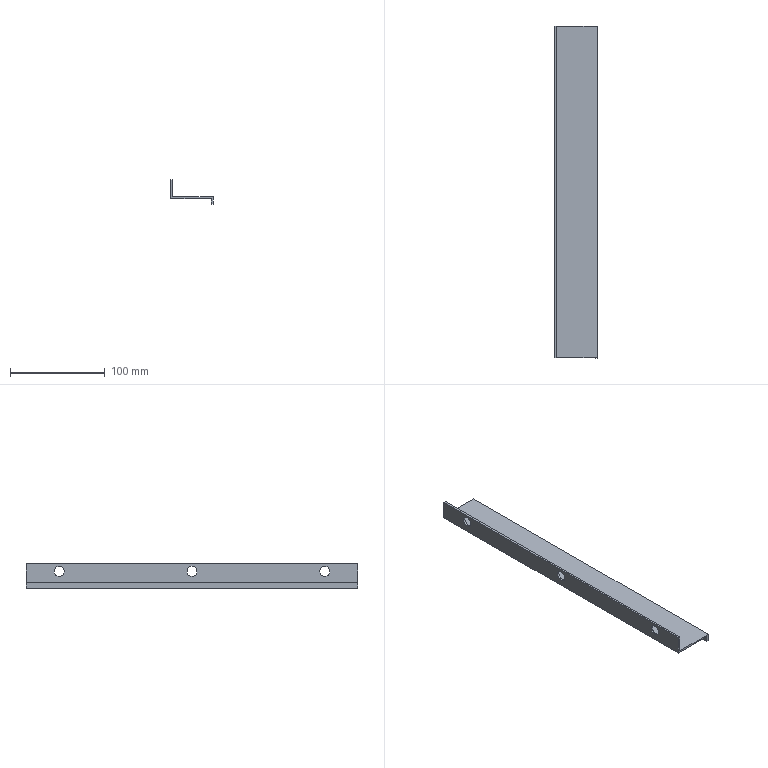Part | SolidWorks | features BaseBody 1 | 1 solid | 16 faces | box 44.5 x 350 x 26 mm | volume 47421 mm3 | plane 10 | cylinder 6 | commonest cylinder face diameters 10.6 x6
STEP:
#1=CARTESIAN_POINT('',(236.946,-4310.973,1968.771));
#2=VERTEX_POINT('',#1);
#3=CARTESIAN_POINT('',(236.946,-4310.973,1958.171));
#4=VERTEX_POINT('',#3);
#5=CARTESIAN_POINT('',(236.946,-4310.973,1963.471));
#6=DIRECTION('',(1.,0.,0.));
#7=DIRECTION('',(0.,0.,-1.));
#8=AXIS2_PLACEMENT_3D('',#5,#6,#7);
#9=CIRCLE('',#8,5.3);
#10=EDGE_CURVE('',#2,#4,#9,.T.);
#11=ORIENTED_EDGE('',*,*,#10,.F.);
#12=CARTESIAN_POINT('',(238.946,-4310.973,1968.771));
#13=VERTEX_POINT('',#12);
#14=CARTESIAN_POINT('',(270.923,-4310.973,1968.771));
#15=DIRECTION('',(1.,0.,0.));
#16=VECTOR('',#15,1000.);
#17=LINE('',#14,#16);
#18=EDGE_CURVE('',#2,#13,#17,.T.);
#19=ORIENTED_EDGE('',*,*,#18,.T.);
#20=CARTESIAN_POINT('',(238.946,-4310.973,1958.171));
#21=VERTEX_POINT('',#20);
#22=CARTESIAN_POINT('',(238.946,-4310.973,1963.471));
#23=DIRECTION('',(-1.,0.,0.));
#24=DIRECTION('',(0.,0.,-1.));
#25=AXIS2_PLACEMENT_3D('',#22,#23,#24);
#26=CIRCLE('',#25,5.3);
#27=EDGE_CURVE('',#21,#13,#26,.T.);
#28=ORIENTED_EDGE('',*,*,#27,.F.);
#29=CARTESIAN_POINT('',(270.923,-4310.973,1958.171));
#30=DIRECTION('',(1.,0.,0.));
#31=VECTOR('',#30,1000.);
#32=LINE('',#29,#31);
#33=EDGE_CURVE('',#4,#21,#32,.T.);
#34=ORIENTED_EDGE('',*,*,#33,.F.);
#35=EDGE_LOOP('',(#11,#19,#28,#34));
#36=FACE_OUTER_BOUND('',#35,.T.);
#37=CARTESIAN_POINT('',(270.923,-4310.973,1963.471));
#38=DIRECTION('',(1.,0.,0.));
#39=DIRECTION('',(0.,0.,-1.));
#40=AXIS2_PLACEMENT_3D('',#37,#38,#39);
#41=CYLINDRICAL_SURFACE('',#40,5.3);
#42=ADVANCED_FACE('',(#36),#41,.F.);
#43=CARTESIAN_POINT('',(236.946,-4030.973,1968.771));
#44=VERTEX_POINT('',#43);
#45=CARTESIAN_POINT('',(236.946,-4030.973,1958.171));
#46=VERTEX_POINT('',#45);
#47=CARTESIAN_POINT('',(236.946,-4030.973,1963.471));
#48=DIRECTION('',(1.,0.,0.));
#49=DIRECTION('',(0.,0.,-1.));
#50=AXIS2_PLACEMENT_3D('',#47,#48,#49);
#51=CIRCLE('',#50,5.3);
#52=EDGE_CURVE('',#44,#46,#51,.T.);
#53=ORIENTED_EDGE('',*,*,#52,.F.);
#54=CARTESIAN_POINT('',(238.946,-4030.973,1968.771));
#55=VERTEX_POINT('',#54);
#56=CARTESIAN_POINT('',(270.923,-4030.973,1968.771));
#57=DIRECTION('',(1.,0.,0.));
#58=VECTOR('',#57,1000.);
#59=LINE('',#56,#58);
#60=EDGE_CURVE('',#44,#55,#59,.T.);
#61=ORIENTED_EDGE('',*,*,#60,.T.);
#62=CARTESIAN_POINT('',(238.946,-4030.973,1958.171));
#63=VERTEX_POINT('',#62);
#64=CARTESIAN_POINT('',(238.946,-4030.973,1963.471));
#65=DIRECTION('',(-1.,0.,0.));
#66=DIRECTION('',(0.,0.,-1.));
#67=AXIS2_PLACEMENT_3D('',#64,#65,#66);
#68=CIRCLE('',#67,5.3);
#69=EDGE_CURVE('',#63,#55,#68,.T.);
#70=ORIENTED_EDGE('',*,*,#69,.F.);
#71=CARTESIAN_POINT('',(270.923,-4030.973,1958.171));
#72=DIRECTION('',(1.,0.,0.));
#73=VECTOR('',#72,1000.);
#74=LINE('',#71,#73);
#75=EDGE_CURVE('',#46,#63,#74,.T.);
#76=ORIENTED_EDGE('',*,*,#75,.F.);
#77=EDGE_LOOP('',(#53,#61,#70,#76));
#78=FACE_OUTER_BOUND('',#77,.T.);
#79=CARTESIAN_POINT('',(270.923,-4030.973,1963.471));
#80=DIRECTION('',(1.,0.,0.));
#81=DIRECTION('',(0.,0.,-1.));
#82=AXIS2_PLACEMENT_3D('',#79,#80,#81);
#83=CYLINDRICAL_SURFACE('',#82,5.3);
#84=ADVANCED_FACE('',(#78),#83,.F.);
#85=CARTESIAN_POINT('',(236.946,-4170.973,1968.771));
#86=VERTEX_POINT('',#85);
#87=CARTESIAN_POINT('',(236.946,-4170.973,1958.171));
#88=VERTEX_POINT('',#87);
#89=CARTESIAN_POINT('',(236.946,-4170.973,1963.471));
#90=DIRECTION('',(1.,0.,0.));
#91=DIRECTION('',(0.,0.,-1.));
#92=AXIS2_PLACEMENT_3D('',#89,#90,#91);
#93=CIRCLE('',#92,5.3);
#94=EDGE_CURVE('',#86,#88,#93,.T.);
#95=ORIENTED_EDGE('',*,*,#94,.F.);
#96=CARTESIAN_POINT('',(238.946,-4170.973,1968.771));
#97=VERTEX_POINT('',#96);
#98=CARTESIAN_POINT('',(270.923,-4170.973,1968.771));
#99=DIRECTION('',(1.,0.,0.));
#100=VECTOR('',#99,1000.);
#101=LINE('',#98,#100);
#102=EDGE_CURVE('',#86,#97,#101,.T.);
#103=ORIENTED_EDGE('',*,*,#102,.T.);
#104=CARTESIAN_POINT('',(238.946,-4170.973,1958.171));
#105=VERTEX_POINT('',#104);
#106=CARTESIAN_POINT('',(238.946,-4170.973,1963.471));
#107=DIRECTION('',(-1.,0.,0.));
#108=DIRECTION('',(0.,0.,-1.));
#109=AXIS2_PLACEMENT_3D('',#106,#107,#108);
#110=CIRCLE('',#109,5.3);
#111=EDGE_CURVE('',#105,#97,#110,.T.);
#112=ORIENTED_EDGE('',*,*,#111,.F.);
#113=CARTESIAN_POINT('',(270.923,-4170.973,1958.171));
#114=DIRECTION('',(1.,0.,0.));
#115=VECTOR('',#114,1000.);
#116=LINE('',#113,#115);
#117=EDGE_CURVE('',#88,#105,#116,.T.);
#118=ORIENTED_EDGE('',*,*,#117,.F.);
#119=EDGE_LOOP('',(#95,#103,#112,#118));
#120=FACE_OUTER_BOUND('',#119,.T.);
#121=CARTESIAN_POINT('',(270.923,-4170.973,1963.471));
#122=DIRECTION('',(1.,0.,0.));
#123=DIRECTION('',(0.,0.,-1.));
#124=AXIS2_PLACEMENT_3D('',#121,#122,#123);
#125=CYLINDRICAL_SURFACE('',#124,5.3);
#126=ADVANCED_FACE('',(#120),#125,.F.);
#127=CARTESIAN_POINT('',(236.946,-3995.973,1951.471));
#128=VERTEX_POINT('',#127);
#129=CARTESIAN_POINT('',(279.446,-3995.973,1951.471));
#130=VERTEX_POINT('',#129);
#131=CARTESIAN_POINT('',(277.446,-3995.973,1951.471));
#132=DIRECTION('',(1.,0.,0.));
#133=VECTOR('',#132,1000.);
#134=LINE('',#131,#133);
#135=EDGE_CURVE('',#128,#130,#134,.T.);
#136=ORIENTED_EDGE('',*,*,#135,.T.);
#137=CARTESIAN_POINT('',(279.446,-4345.973,1951.471));
#138=VERTEX_POINT('',#137);
#139=CARTESIAN_POINT('',(279.446,-3995.973,1951.471));
#140=DIRECTION('',(0.,-1.,0.));
#141=VECTOR('',#140,1000.);
#142=LINE('',#139,#141);
#143=EDGE_CURVE('',#130,#138,#142,.T.);
#144=ORIENTED_EDGE('',*,*,#143,.T.);
#145=CARTESIAN_POINT('',(236.946,-4345.973,1951.471));
#146=VERTEX_POINT('',#145);
#147=CARTESIAN_POINT('',(277.446,-4345.973,1951.471));
#148=DIRECTION('',(-1.,0.,0.));
#149=VECTOR('',#148,1000.);
#150=LINE('',#147,#149);
#151=EDGE_CURVE('',#138,#146,#150,.T.);
#152=ORIENTED_EDGE('',*,*,#151,.T.);
#153=CARTESIAN_POINT('',(236.946,-3995.973,1951.471));
#154=DIRECTION('',(0.,1.,0.));
#155=VECTOR('',#154,1000.);
#156=LINE('',#153,#155);
#157=EDGE_CURVE('',#146,#128,#156,.T.);
#158=ORIENTED_EDGE('',*,*,#157,.T.);
#159=EDGE_LOOP('',(#136,#144,#152,#158));
#160=FACE_OUTER_BOUND('',#159,.T.);
#161=CARTESIAN_POINT('',(277.446,-3995.973,1951.471));
#162=DIRECTION('',(0.,0.,-1.));
#163=DIRECTION('',(-1.,0.,0.));
#164=AXIS2_PLACEMENT_3D('',#161,#162,#163);
#165=PLANE('',#164);
#166=ADVANCED_FACE('',(#160),#165,.T.);
#167=CARTESIAN_POINT('',(279.446,-3995.973,1945.471));
#168=VERTEX_POINT('',#167);
#169=CARTESIAN_POINT('',(279.446,-3995.973,1945.471));
#170=DIRECTION('',(0.,0.,-1.));
#171=VECTOR('',#170,1000.);
#172=LINE('',#169,#171);
#173=EDGE_CURVE('',#130,#168,#172,.T.);
#174=ORIENTED_EDGE('',*,*,#173,.T.);
#175=CARTESIAN_POINT('',(279.446,-4345.973,1945.471));
#176=VERTEX_POINT('',#175);
#177=CARTESIAN_POINT('',(279.446,-3995.973,1945.471));
#178=DIRECTION('',(0.,-1.,0.));
#179=VECTOR('',#178,1000.);
#180=LINE('',#177,#179);
#181=EDGE_CURVE('',#168,#176,#180,.T.);
#182=ORIENTED_EDGE('',*,*,#181,.T.);
#183=CARTESIAN_POINT('',(279.446,-4345.973,1945.471));
#184=DIRECTION('',(0.,0.,1.));
#185=VECTOR('',#184,1000.);
#186=LINE('',#183,#185);
#187=EDGE_CURVE('',#176,#138,#186,.T.);
#188=ORIENTED_EDGE('',*,*,#187,.T.);
#189=ORIENTED_EDGE('',*,*,#143,.F.);
#190=EDGE_LOOP('',(#174,#182,#188,#189));
#191=FACE_OUTER_BOUND('',#190,.T.);
#192=CARTESIAN_POINT('',(279.446,-3995.973,1945.471));
#193=DIRECTION('',(-1.,0.,0.));
#194=DIRECTION('',(0.,0.,1.));
#195=AXIS2_PLACEMENT_3D('',#192,#193,#194);
#196=PLANE('',#195);
#197=ADVANCED_FACE('',(#191),#196,.T.);
#198=CARTESIAN_POINT('',(236.946,-3995.973,1971.471));
#199=VERTEX_POINT('',#198);
#200=CARTESIAN_POINT('',(236.946,-3995.973,1956.835));
#201=DIRECTION('',(0.,0.,1.));
#202=VECTOR('',#201,1000.);
#203=LINE('',#200,#202);
#204=EDGE_CURVE('',#128,#199,#203,.T.);
#205=ORIENTED_EDGE('',*,*,#204,.T.);
#206=CARTESIAN_POINT('',(238.946,-3995.973,1971.471));
#207=VERTEX_POINT('',#206);
#208=CARTESIAN_POINT('',(271.559,-3995.973,1971.471));
#209=DIRECTION('',(1.,0.,0.));
#210=VECTOR('',#209,1000.);
#211=LINE('',#208,#210);
#212=EDGE_CURVE('',#199,#207,#211,.T.);
#213=ORIENTED_EDGE('',*,*,#212,.T.);
#214=CARTESIAN_POINT('',(238.946,-3995.973,1953.471));
#215=VERTEX_POINT('',#214);
#216=CARTESIAN_POINT('',(238.946,-3995.973,1956.835));
#217=DIRECTION('',(0.,0.,-1.));
#218=VECTOR('',#217,1000.);
#219=LINE('',#216,#218);
#220=EDGE_CURVE('',#207,#215,#219,.T.);
#221=ORIENTED_EDGE('',*,*,#220,.T.);
#222=CARTESIAN_POINT('',(281.446,-3995.973,1953.471));
#223=VERTEX_POINT('',#222);
#224=CARTESIAN_POINT('',(271.559,-3995.973,1953.471));
#225=DIRECTION('',(1.,0.,0.));
#226=VECTOR('',#225,1000.);
#227=LINE('',#224,#226);
#228=EDGE_CURVE('',#215,#223,#227,.T.);
#229=ORIENTED_EDGE('',*,*,#228,.T.);
#230=CARTESIAN_POINT('',(281.446,-3995.973,1945.471));
#231=VERTEX_POINT('',#230);
#232=CARTESIAN_POINT('',(281.446,-3995.973,1956.835));
#233=DIRECTION('',(0.,0.,-1.));
#234=VECTOR('',#233,1000.);
#235=LINE('',#232,#234);
#236=EDGE_CURVE('',#223,#231,#235,.T.);
#237=ORIENTED_EDGE('',*,*,#236,.T.);
#238=CARTESIAN_POINT('',(271.559,-3995.973,1945.471));
#239=DIRECTION('',(-1.,0.,0.));
#240=VECTOR('',#239,1000.);
#241=LINE('',#238,#240);
#242=EDGE_CURVE('',#231,#168,#241,.T.);
#243=ORIENTED_EDGE('',*,*,#242,.T.);
#244=ORIENTED_EDGE('',*,*,#173,.F.);
#245=ORIENTED_EDGE('',*,*,#135,.F.);
#246=EDGE_LOOP('',(#205,#213,#221,#229,#237,#243,#244,#245));
#247=FACE_OUTER_BOUND('',#246,.T.);
#248=CARTESIAN_POINT('',(271.559,-3995.973,1956.835));
#249=DIRECTION('',(0.,1.,0.));
#250=DIRECTION('',(0.,0.,1.));
#251=AXIS2_PLACEMENT_3D('',#248,#249,#250);
#252=PLANE('',#251);
#253=ADVANCED_FACE('',(#247),#252,.T.);
#254=ORIENTED_EDGE('',*,*,#204,.F.);
#255=ORIENTED_EDGE('',*,*,#157,.F.);
#256=CARTESIAN_POINT('',(236.946,-4345.973,1971.471));
#257=VERTEX_POINT('',#256);
#258=CARTESIAN_POINT('',(236.946,-4345.973,1951.471));
#259=DIRECTION('',(0.,0.,1.));
#260=VECTOR('',#259,1000.);
#261=LINE('',#258,#260);
#262=EDGE_CURVE('',#146,#257,#261,.T.);
#263=ORIENTED_EDGE('',*,*,#262,.T.);
#264=CARTESIAN_POINT('',(236.946,-3995.973,1971.471));
#265=DIRECTION('',(0.,1.,0.));
#266=VECTOR('',#265,1000.);
#267=LINE('',#264,#266);
#268=EDGE_CURVE('',#257,#199,#267,.T.);
#269=ORIENTED_EDGE('',*,*,#268,.T.);
#270=EDGE_LOOP('',(#254,#255,#263,#269));
#271=FACE_OUTER_BOUND('',#270,.T.);
#272=CARTESIAN_POINT('',(236.946,-4310.973,1963.471));
#273=DIRECTION('',(1.,0.,0.));
#274=DIRECTION('',(0.,0.,-1.));
#275=AXIS2_PLACEMENT_3D('',#272,#273,#274);
#276=CIRCLE('',#275,5.3);
#277=EDGE_CURVE('',#4,#2,#276,.T.);
#278=ORIENTED_EDGE('',*,*,#277,.T.);
#279=ORIENTED_EDGE('',*,*,#10,.T.);
#280=EDGE_LOOP('',(#278,#279));
#281=FACE_BOUND('',#280,.T.);
#282=CARTESIAN_POINT('',(236.946,-4030.973,1963.471));
#283=DIRECTION('',(1.,0.,0.));
#284=DIRECTION('',(0.,0.,-1.));
#285=AXIS2_PLACEMENT_3D('',#282,#283,#284);
#286=CIRCLE('',#285,5.3);
#287=EDGE_CURVE('',#46,#44,#286,.T.);
#288=ORIENTED_EDGE('',*,*,#287,.T.);
#289=ORIENTED_EDGE('',*,*,#52,.T.);
#290=EDGE_LOOP('',(#288,#289));
#291=FACE_BOUND('',#290,.T.);
#292=CARTESIAN_POINT('',(236.946,-4170.973,1963.471));
#293=DIRECTION('',(1.,0.,0.));
#294=DIRECTION('',(0.,0.,-1.));
#295=AXIS2_PLACEMENT_3D('',#292,#293,#294);
#296=CIRCLE('',#295,5.3);
#297=EDGE_CURVE('',#88,#86,#296,.T.);
#298=ORIENTED_EDGE('',*,*,#297,.T.);
#299=ORIENTED_EDGE('',*,*,#94,.T.);
#300=EDGE_LOOP('',(#298,#299));
#301=FACE_BOUND('',#300,.T.);
#302=CARTESIAN_POINT('',(236.946,-3995.973,1951.471));
#303=DIRECTION('',(-1.,0.,0.));
#304=DIRECTION('',(0.,0.,1.));
#305=AXIS2_PLACEMENT_3D('',#302,#303,#304);
#306=PLANE('',#305);
#307=ADVANCED_FACE('',(#271,#281,#291,#301),#306,.T.);
#308=CARTESIAN_POINT('',(238.946,-4345.973,1971.471));
#309=VERTEX_POINT('',#308);
#310=CARTESIAN_POINT('',(238.946,-4345.973,1953.471));
#311=VERTEX_POINT('',#310);
#312=CARTESIAN_POINT('',(238.946,-4345.973,1956.835));
#313=DIRECTION('',(0.,0.,-1.));
#314=VECTOR('',#313,1000.);
#315=LINE('',#312,#314);
#316=EDGE_CURVE('',#309,#311,#315,.T.);
#317=ORIENTED_EDGE('',*,*,#316,.F.);
#318=CARTESIAN_POINT('',(213.059,-4345.973,1971.471));
#319=DIRECTION('',(1.,0.,0.));
#320=VECTOR('',#319,1000.);
#321=LINE('',#318,#320);
#322=EDGE_CURVE('',#257,#309,#321,.T.);
#323=ORIENTED_EDGE('',*,*,#322,.F.);
#324=ORIENTED_EDGE('',*,*,#262,.F.);
#325=ORIENTED_EDGE('',*,*,#151,.F.);
#326=ORIENTED_EDGE('',*,*,#187,.F.);
#327=CARTESIAN_POINT('',(281.446,-4345.973,1945.471));
#328=VERTEX_POINT('',#327);
#329=CARTESIAN_POINT('',(213.059,-4345.973,1945.471));
#330=DIRECTION('',(-1.,0.,0.));
#331=VECTOR('',#330,1000.);
#332=LINE('',#329,#331);
#333=EDGE_CURVE('',#328,#176,#332,.T.);
#334=ORIENTED_EDGE('',*,*,#333,.F.);
#335=CARTESIAN_POINT('',(281.446,-4345.973,1953.471));
#336=VERTEX_POINT('',#335);
#337=CARTESIAN_POINT('',(281.446,-4345.973,1956.835));
#338=DIRECTION('',(0.,0.,-1.));
#339=VECTOR('',#338,1000.);
#340=LINE('',#337,#339);
#341=EDGE_CURVE('',#336,#328,#340,.T.);
#342=ORIENTED_EDGE('',*,*,#341,.F.);
#343=CARTESIAN_POINT('',(213.059,-4345.973,1953.471));
#344=DIRECTION('',(1.,0.,0.));
#345=VECTOR('',#344,1000.);
#346=LINE('',#343,#345);
#347=EDGE_CURVE('',#311,#336,#346,.T.);
#348=ORIENTED_EDGE('',*,*,#347,.F.);
#349=EDGE_LOOP('',(#317,#323,#324,#325,#326,#334,#342,#348));
#350=FACE_OUTER_BOUND('',#349,.T.);
#351=CARTESIAN_POINT('',(213.059,-4345.973,1956.835));
#352=DIRECTION('',(0.,1.,0.));
#353=DIRECTION('',(0.,0.,1.));
#354=AXIS2_PLACEMENT_3D('',#351,#352,#353);
#355=PLANE('',#354);
#356=ADVANCED_FACE('',(#350),#355,.F.);
#357=ORIENTED_EDGE('',*,*,#242,.F.);
#358=CARTESIAN_POINT('',(281.446,-3995.973,1945.471));
#359=DIRECTION('',(0.,-1.,0.));
#360=VECTOR('',#359,1000.);
#361=LINE('',#358,#360);
#362=EDGE_CURVE('',#231,#328,#361,.T.);
#363=ORIENTED_EDGE('',*,*,#362,.T.);
#364=ORIENTED_EDGE('',*,*,#333,.T.);
#365=ORIENTED_EDGE('',*,*,#181,.F.);
#366=EDGE_LOOP('',(#357,#363,#364,#365));
#367=FACE_OUTER_BOUND('',#366,.T.);
#368=CARTESIAN_POINT('',(279.446,-3995.973,1945.471));
#369=DIRECTION('',(0.,0.,-1.));
#370=DIRECTION('',(-1.,0.,0.));
#371=AXIS2_PLACEMENT_3D('',#368,#369,#370);
#372=PLANE('',#371);
#373=ADVANCED_FACE('',(#367),#372,.T.);
#374=ORIENTED_EDGE('',*,*,#212,.F.);
#375=ORIENTED_EDGE('',*,*,#268,.F.);
#376=ORIENTED_EDGE('',*,*,#322,.T.);
#377=CARTESIAN_POINT('',(238.946,-3995.973,1971.471));
#378=DIRECTION('',(0.,1.,0.));
#379=VECTOR('',#378,1000.);
#380=LINE('',#377,#379);
#381=EDGE_CURVE('',#309,#207,#380,.T.);
#382=ORIENTED_EDGE('',*,*,#381,.T.);
#383=EDGE_LOOP('',(#374,#375,#376,#382));
#384=FACE_OUTER_BOUND('',#383,.T.);
#385=CARTESIAN_POINT('',(266.946,-3995.973,1971.471));
#386=DIRECTION('',(0.,0.,1.));
#387=DIRECTION('',(1.,0.,0.));
#388=AXIS2_PLACEMENT_3D('',#385,#386,#387);
#389=PLANE('',#388);
#390=ADVANCED_FACE('',(#384),#389,.T.);
#391=ORIENTED_EDGE('',*,*,#236,.F.);
#392=CARTESIAN_POINT('',(281.446,-3995.973,1953.471));
#393=DIRECTION('',(0.,-1.,0.));
#394=VECTOR('',#393,1000.);
#395=LINE('',#392,#394);
#396=EDGE_CURVE('',#223,#336,#395,.T.);
#397=ORIENTED_EDGE('',*,*,#396,.T.);
#398=ORIENTED_EDGE('',*,*,#341,.T.);
#399=ORIENTED_EDGE('',*,*,#362,.F.);
#400=EDGE_LOOP('',(#391,#397,#398,#399));
#401=FACE_OUTER_BOUND('',#400,.T.);
#402=CARTESIAN_POINT('',(281.446,-3995.973,1953.471));
#403=DIRECTION('',(1.,0.,0.));
#404=DIRECTION('',(0.,0.,-1.));
#405=AXIS2_PLACEMENT_3D('',#402,#403,#404);
#406=PLANE('',#405);
#407=ADVANCED_FACE('',(#401),#406,.T.);
#408=ORIENTED_EDGE('',*,*,#228,.F.);
#409=CARTESIAN_POINT('',(238.946,-3995.973,1953.471));
#410=DIRECTION('',(0.,-1.,0.));
#411=VECTOR('',#410,1000.);
#412=LINE('',#409,#411);
#413=EDGE_CURVE('',#215,#311,#412,.T.);
#414=ORIENTED_EDGE('',*,*,#413,.T.);
#415=ORIENTED_EDGE('',*,*,#347,.T.);
#416=ORIENTED_EDGE('',*,*,#396,.F.);
#417=EDGE_LOOP('',(#408,#414,#415,#416));
#418=FACE_OUTER_BOUND('',#417,.T.);
#419=CARTESIAN_POINT('',(271.446,-3995.973,1953.471));
#420=DIRECTION('',(0.,0.,1.));
#421=DIRECTION('',(1.,0.,0.));
#422=AXIS2_PLACEMENT_3D('',#419,#420,#421);
#423=PLANE('',#422);
#424=ADVANCED_FACE('',(#418),#423,.T.);
#425=ORIENTED_EDGE('',*,*,#220,.F.);
#426=ORIENTED_EDGE('',*,*,#381,.F.);
#427=ORIENTED_EDGE('',*,*,#316,.T.);
#428=ORIENTED_EDGE('',*,*,#413,.F.);
#429=EDGE_LOOP('',(#425,#426,#427,#428));
#430=FACE_OUTER_BOUND('',#429,.T.);
#431=ORIENTED_EDGE('',*,*,#27,.T.);
#432=CARTESIAN_POINT('',(238.946,-4310.973,1963.471));
#433=DIRECTION('',(-1.,0.,0.));
#434=DIRECTION('',(0.,0.,-1.));
#435=AXIS2_PLACEMENT_3D('',#432,#433,#434);
#436=CIRCLE('',#435,5.3);
#437=EDGE_CURVE('',#13,#21,#436,.T.);
#438=ORIENTED_EDGE('',*,*,#437,.T.);
#439=EDGE_LOOP('',(#431,#438));
#440=FACE_BOUND('',#439,.T.);
#441=ORIENTED_EDGE('',*,*,#69,.T.);
#442=CARTESIAN_POINT('',(238.946,-4030.973,1963.471));
#443=DIRECTION('',(-1.,0.,0.));
#444=DIRECTION('',(0.,0.,-1.));
#445=AXIS2_PLACEMENT_3D('',#442,#443,#444);
#446=CIRCLE('',#445,5.3);
#447=EDGE_CURVE('',#55,#63,#446,.T.);
#448=ORIENTED_EDGE('',*,*,#447,.T.);
#449=EDGE_LOOP('',(#441,#448));
#450=FACE_BOUND('',#449,.T.);
#451=ORIENTED_EDGE('',*,*,#111,.T.);
#452=CARTESIAN_POINT('',(238.946,-4170.973,1963.471));
#453=DIRECTION('',(-1.,0.,0.));
#454=DIRECTION('',(0.,0.,-1.));
#455=AXIS2_PLACEMENT_3D('',#452,#453,#454);
#456=CIRCLE('',#455,5.3);
#457=EDGE_CURVE('',#97,#105,#456,.T.);
#458=ORIENTED_EDGE('',*,*,#457,.T.);
#459=EDGE_LOOP('',(#451,#458));
#460=FACE_BOUND('',#459,.T.);
#461=CARTESIAN_POINT('',(238.946,-3995.973,1971.471));
#462=DIRECTION('',(1.,0.,0.));
#463=DIRECTION('',(0.,0.,-1.));
#464=AXIS2_PLACEMENT_3D('',#461,#462,#463);
#465=PLANE('',#464);
#466=ADVANCED_FACE('',(#430,#440,#450,#460),#465,.T.);
#467=ORIENTED_EDGE('',*,*,#18,.F.);
#468=ORIENTED_EDGE('',*,*,#277,.F.);
#469=ORIENTED_EDGE('',*,*,#33,.T.);
#470=ORIENTED_EDGE('',*,*,#437,.F.);
#471=EDGE_LOOP('',(#467,#468,#469,#470));
#472=FACE_OUTER_BOUND('',#471,.T.);
#473=CARTESIAN_POINT('',(270.923,-4310.973,1963.471));
#474=DIRECTION('',(1.,0.,0.));
#475=DIRECTION('',(0.,0.,-1.));
#476=AXIS2_PLACEMENT_3D('',#473,#474,#475);
#477=CYLINDRICAL_SURFACE('',#476,5.3);
#478=ADVANCED_FACE('',(#472),#477,.F.);
#479=ORIENTED_EDGE('',*,*,#60,.F.);
#480=ORIENTED_EDGE('',*,*,#287,.F.);
#481=ORIENTED_EDGE('',*,*,#75,.T.);
#482=ORIENTED_EDGE('',*,*,#447,.F.);
#483=EDGE_LOOP('',(#479,#480,#481,#482));
#484=FACE_OUTER_BOUND('',#483,.T.);
#485=CARTESIAN_POINT('',(270.923,-4030.973,1963.471));
#486=DIRECTION('',(1.,0.,0.));
#487=DIRECTION('',(0.,0.,-1.));
#488=AXIS2_PLACEMENT_3D('',#485,#486,#487);
#489=CYLINDRICAL_SURFACE('',#488,5.3);
#490=ADVANCED_FACE('',(#484),#489,.F.);
#491=ORIENTED_EDGE('',*,*,#102,.F.);
#492=ORIENTED_EDGE('',*,*,#297,.F.);
#493=ORIENTED_EDGE('',*,*,#117,.T.);
#494=ORIENTED_EDGE('',*,*,#457,.F.);
#495=EDGE_LOOP('',(#491,#492,#493,#494));
#496=FACE_OUTER_BOUND('',#495,.T.);
#497=CARTESIAN_POINT('',(270.923,-4170.973,1963.471));
#498=DIRECTION('',(1.,0.,0.));
#499=DIRECTION('',(0.,0.,-1.));
#500=AXIS2_PLACEMENT_3D('',#497,#498,#499);
#501=CYLINDRICAL_SURFACE('',#500,5.3);
#502=ADVANCED_FACE('',(#496),#501,.F.);
#503=CLOSED_SHELL('',(#42,#84,#126,#166,#197,#253,#307,#356,#373,#390,#407,#424,#466,#478,#490,#502));
#504=MANIFOLD_SOLID_BREP('',#503);
#505=CARTESIAN_POINT('',(0.,0.,0.));
#506=DIRECTION('',(0.,0.,1.));
#507=DIRECTION('',(1.,0.,0.));
#508=AXIS2_PLACEMENT_3D('',#505,#506,#507);
#509=(LENGTH_UNIT()NAMED_UNIT(*)SI_UNIT(.MILLI.,.METRE.));
#510=UNCERTAINTY_MEASURE_WITH_UNIT(LENGTH_MEASURE(0.00001),#509,'','');
#511=(NAMED_UNIT(*)PLANE_ANGLE_UNIT()SI_UNIT($,.RADIAN.));
#512=(NAMED_UNIT(*)SI_UNIT($,.STERADIAN.)SOLID_ANGLE_UNIT());
#513=(GEOMETRIC_REPRESENTATION_CONTEXT(3)GLOBAL_UNCERTAINTY_ASSIGNED_CONTEXT((#510))GLOBAL_UNIT_ASSIGNED_CONTEXT((#509,#511,#512))REPRESENTATION_CONTEXT('',''));
#514=ADVANCED_BREP_SHAPE_REPRESENTATION('',(#504,#508),#513);